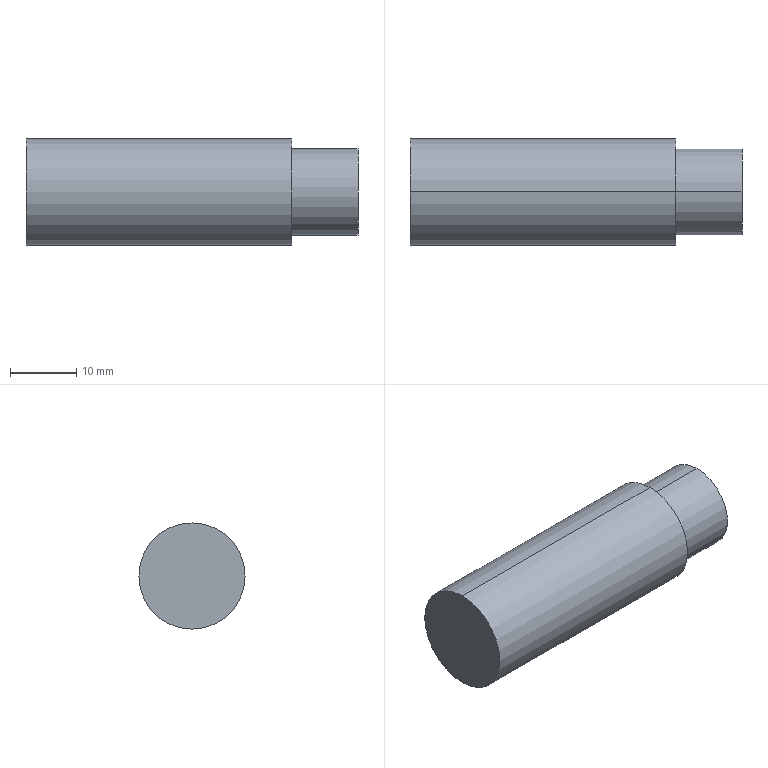Part | SolidWorks | features Revolution 1 | 1 solid | 7 faces | box 50 x 16 x 16 mm | volume 9370 mm3 | cylinder 4 | plane 3 | commonest cylinder face diameters 13 x2 16 x2
STEP:
#1=CARTESIAN_POINT('',(50.,0.,6.5));
#2=VERTEX_POINT('',#1);
#3=CARTESIAN_POINT('',(50.,0.,-6.5));
#4=VERTEX_POINT('',#3);
#5=CARTESIAN_POINT('',(50.,0.,0.));
#6=DIRECTION('',(-1.,0.,0.));
#7=DIRECTION('',(0.,0.,1.));
#8=AXIS2_PLACEMENT_3D('',#5,#6,#7);
#9=CIRCLE('',#8,6.5);
#10=EDGE_CURVE('',#2,#4,#9,.T.);
#11=ORIENTED_EDGE('',*,*,#10,.T.);
#12=CARTESIAN_POINT('',(40.,0.,-6.5));
#13=VERTEX_POINT('',#12);
#14=CARTESIAN_POINT('',(0.,0.,-6.5));
#15=DIRECTION('',(-1.,0.,0.));
#16=VECTOR('',#15,1000.);
#17=LINE('',#14,#16);
#18=EDGE_CURVE('',#4,#13,#17,.T.);
#19=ORIENTED_EDGE('',*,*,#18,.T.);
#20=CARTESIAN_POINT('',(40.,0.,6.5));
#21=VERTEX_POINT('',#20);
#22=CARTESIAN_POINT('',(40.,0.,0.));
#23=DIRECTION('',(-1.,0.,0.));
#24=DIRECTION('',(0.,0.,1.));
#25=AXIS2_PLACEMENT_3D('',#22,#23,#24);
#26=CIRCLE('',#25,6.5);
#27=EDGE_CURVE('',#21,#13,#26,.T.);
#28=ORIENTED_EDGE('',*,*,#27,.F.);
#29=CARTESIAN_POINT('',(0.,0.,6.5));
#30=DIRECTION('',(-1.,0.,0.));
#31=VECTOR('',#30,1000.);
#32=LINE('',#29,#31);
#33=EDGE_CURVE('',#2,#21,#32,.T.);
#34=ORIENTED_EDGE('',*,*,#33,.F.);
#35=EDGE_LOOP('',(#11,#19,#28,#34));
#36=FACE_OUTER_BOUND('',#35,.T.);
#37=CARTESIAN_POINT('',(0.,0.,0.));
#38=DIRECTION('',(-1.,0.,0.));
#39=DIRECTION('',(0.,0.,1.));
#40=AXIS2_PLACEMENT_3D('',#37,#38,#39);
#41=CYLINDRICAL_SURFACE('',#40,6.5);
#42=ADVANCED_FACE('',(#36),#41,.T.);
#43=CARTESIAN_POINT('',(40.,0.,8.));
#44=VERTEX_POINT('',#43);
#45=CARTESIAN_POINT('',(40.,0.,-8.));
#46=VERTEX_POINT('',#45);
#47=CARTESIAN_POINT('',(40.,0.,0.));
#48=DIRECTION('',(-1.,0.,0.));
#49=DIRECTION('',(0.,0.,1.));
#50=AXIS2_PLACEMENT_3D('',#47,#48,#49);
#51=CIRCLE('',#50,8.);
#52=EDGE_CURVE('',#44,#46,#51,.T.);
#53=ORIENTED_EDGE('',*,*,#52,.T.);
#54=CARTESIAN_POINT('',(0.,0.,-8.));
#55=VERTEX_POINT('',#54);
#56=CARTESIAN_POINT('',(0.,0.,-8.));
#57=DIRECTION('',(-1.,0.,0.));
#58=VECTOR('',#57,1000.);
#59=LINE('',#56,#58);
#60=EDGE_CURVE('',#46,#55,#59,.T.);
#61=ORIENTED_EDGE('',*,*,#60,.T.);
#62=CARTESIAN_POINT('',(0.,0.,8.));
#63=VERTEX_POINT('',#62);
#64=CARTESIAN_POINT('',(0.,0.,0.));
#65=DIRECTION('',(-1.,0.,0.));
#66=DIRECTION('',(0.,0.,1.));
#67=AXIS2_PLACEMENT_3D('',#64,#65,#66);
#68=CIRCLE('',#67,8.);
#69=EDGE_CURVE('',#63,#55,#68,.T.);
#70=ORIENTED_EDGE('',*,*,#69,.F.);
#71=CARTESIAN_POINT('',(0.,0.,8.));
#72=DIRECTION('',(-1.,0.,0.));
#73=VECTOR('',#72,1000.);
#74=LINE('',#71,#73);
#75=EDGE_CURVE('',#44,#63,#74,.T.);
#76=ORIENTED_EDGE('',*,*,#75,.F.);
#77=EDGE_LOOP('',(#53,#61,#70,#76));
#78=FACE_OUTER_BOUND('',#77,.T.);
#79=CARTESIAN_POINT('',(0.,0.,0.));
#80=DIRECTION('',(-1.,0.,0.));
#81=DIRECTION('',(0.,0.,1.));
#82=AXIS2_PLACEMENT_3D('',#79,#80,#81);
#83=CYLINDRICAL_SURFACE('',#82,8.);
#84=ADVANCED_FACE('',(#78),#83,.T.);
#85=ORIENTED_EDGE('',*,*,#69,.T.);
#86=CARTESIAN_POINT('',(0.,0.,0.));
#87=DIRECTION('',(-1.,0.,0.));
#88=DIRECTION('',(0.,0.,1.));
#89=AXIS2_PLACEMENT_3D('',#86,#87,#88);
#90=CIRCLE('',#89,8.);
#91=EDGE_CURVE('',#55,#63,#90,.T.);
#92=ORIENTED_EDGE('',*,*,#91,.T.);
#93=EDGE_LOOP('',(#85,#92));
#94=FACE_OUTER_BOUND('',#93,.T.);
#95=CARTESIAN_POINT('',(0.,0.,0.));
#96=DIRECTION('',(1.,0.,0.));
#97=DIRECTION('',(0.,0.,-1.));
#98=AXIS2_PLACEMENT_3D('',#95,#96,#97);
#99=PLANE('',#98);
#100=ADVANCED_FACE('',(#94),#99,.F.);
#101=ORIENTED_EDGE('',*,*,#60,.F.);
#102=CARTESIAN_POINT('',(40.,0.,0.));
#103=DIRECTION('',(-1.,0.,0.));
#104=DIRECTION('',(0.,0.,1.));
#105=AXIS2_PLACEMENT_3D('',#102,#103,#104);
#106=CIRCLE('',#105,8.);
#107=EDGE_CURVE('',#46,#44,#106,.T.);
#108=ORIENTED_EDGE('',*,*,#107,.T.);
#109=ORIENTED_EDGE('',*,*,#75,.T.);
#110=ORIENTED_EDGE('',*,*,#91,.F.);
#111=EDGE_LOOP('',(#101,#108,#109,#110));
#112=FACE_OUTER_BOUND('',#111,.T.);
#113=CARTESIAN_POINT('',(0.,0.,0.));
#114=DIRECTION('',(-1.,0.,0.));
#115=DIRECTION('',(0.,0.,1.));
#116=AXIS2_PLACEMENT_3D('',#113,#114,#115);
#117=CYLINDRICAL_SURFACE('',#116,8.);
#118=ADVANCED_FACE('',(#112),#117,.T.);
#119=ORIENTED_EDGE('',*,*,#52,.F.);
#120=ORIENTED_EDGE('',*,*,#107,.F.);
#121=EDGE_LOOP('',(#119,#120));
#122=FACE_OUTER_BOUND('',#121,.T.);
#123=ORIENTED_EDGE('',*,*,#27,.T.);
#124=CARTESIAN_POINT('',(40.,0.,0.));
#125=DIRECTION('',(-1.,0.,0.));
#126=DIRECTION('',(0.,0.,1.));
#127=AXIS2_PLACEMENT_3D('',#124,#125,#126);
#128=CIRCLE('',#127,6.5);
#129=EDGE_CURVE('',#13,#21,#128,.T.);
#130=ORIENTED_EDGE('',*,*,#129,.T.);
#131=EDGE_LOOP('',(#123,#130));
#132=FACE_BOUND('',#131,.T.);
#133=CARTESIAN_POINT('',(40.,8.,0.));
#134=DIRECTION('',(-1.,0.,0.));
#135=DIRECTION('',(0.,0.,1.));
#136=AXIS2_PLACEMENT_3D('',#133,#134,#135);
#137=PLANE('',#136);
#138=ADVANCED_FACE('',(#122,#132),#137,.F.);
#139=ORIENTED_EDGE('',*,*,#18,.F.);
#140=CARTESIAN_POINT('',(50.,0.,0.));
#141=DIRECTION('',(-1.,0.,0.));
#142=DIRECTION('',(0.,0.,1.));
#143=AXIS2_PLACEMENT_3D('',#140,#141,#142);
#144=CIRCLE('',#143,6.5);
#145=EDGE_CURVE('',#4,#2,#144,.T.);
#146=ORIENTED_EDGE('',*,*,#145,.T.);
#147=ORIENTED_EDGE('',*,*,#33,.T.);
#148=ORIENTED_EDGE('',*,*,#129,.F.);
#149=EDGE_LOOP('',(#139,#146,#147,#148));
#150=FACE_OUTER_BOUND('',#149,.T.);
#151=CARTESIAN_POINT('',(0.,0.,0.));
#152=DIRECTION('',(-1.,0.,0.));
#153=DIRECTION('',(0.,0.,1.));
#154=AXIS2_PLACEMENT_3D('',#151,#152,#153);
#155=CYLINDRICAL_SURFACE('',#154,6.5);
#156=ADVANCED_FACE('',(#150),#155,.T.);
#157=ORIENTED_EDGE('',*,*,#10,.F.);
#158=ORIENTED_EDGE('',*,*,#145,.F.);
#159=EDGE_LOOP('',(#157,#158));
#160=FACE_OUTER_BOUND('',#159,.T.);
#161=CARTESIAN_POINT('',(50.,6.5,0.));
#162=DIRECTION('',(-1.,0.,0.));
#163=DIRECTION('',(0.,0.,1.));
#164=AXIS2_PLACEMENT_3D('',#161,#162,#163);
#165=PLANE('',#164);
#166=ADVANCED_FACE('',(#160),#165,.F.);
#167=CLOSED_SHELL('',(#42,#84,#100,#118,#138,#156,#166));
#168=MANIFOLD_SOLID_BREP('',#167);
#169=CARTESIAN_POINT('',(0.,0.,0.));
#170=DIRECTION('',(0.,0.,1.));
#171=DIRECTION('',(1.,0.,0.));
#172=AXIS2_PLACEMENT_3D('',#169,#170,#171);
#173=(LENGTH_UNIT()NAMED_UNIT(*)SI_UNIT(.MILLI.,.METRE.));
#174=UNCERTAINTY_MEASURE_WITH_UNIT(LENGTH_MEASURE(0.00001),#173,'','');
#175=(NAMED_UNIT(*)PLANE_ANGLE_UNIT()SI_UNIT($,.RADIAN.));
#176=(NAMED_UNIT(*)SI_UNIT($,.STERADIAN.)SOLID_ANGLE_UNIT());
#177=(GEOMETRIC_REPRESENTATION_CONTEXT(3)GLOBAL_UNCERTAINTY_ASSIGNED_CONTEXT((#174))GLOBAL_UNIT_ASSIGNED_CONTEXT((#173,#175,#176))REPRESENTATION_CONTEXT('',''));
#178=ADVANCED_BREP_SHAPE_REPRESENTATION('',(#168,#172),#177);